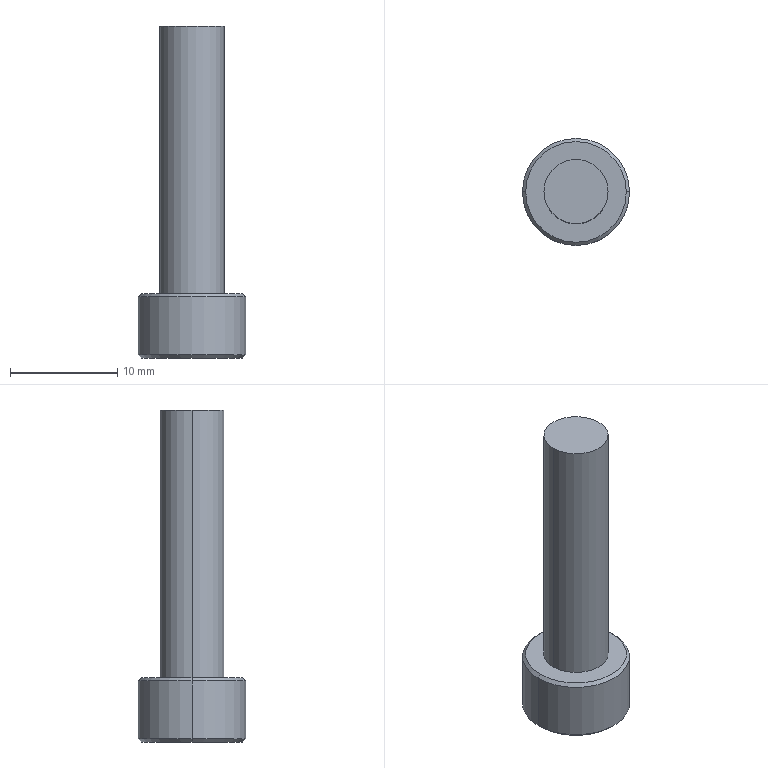Part | SolidWorks | features ICE 2, Chamfer 1, Extrusion 1 | 1 solid | 18 faces | box 10 x 10 x 31 mm | volume 1129 mm3 | plane 10 | cone 4 | cylinder 4 | commonest cylinder face diameters 6 x2 10 x2
STEP:
#1=CARTESIAN_POINT('',(4.7,0.,6.));
#2=VERTEX_POINT('',#1);
#3=CARTESIAN_POINT('',(-4.7,0.,6.));
#4=VERTEX_POINT('',#3);
#5=CARTESIAN_POINT('',(0.,0.,6.));
#6=DIRECTION('',(0.,0.,1.));
#7=DIRECTION('',(1.,0.,0.));
#8=AXIS2_PLACEMENT_3D('',#5,#6,#7);
#9=CIRCLE('',#8,4.7);
#10=EDGE_CURVE('',#2,#4,#9,.T.);
#11=ORIENTED_EDGE('',*,*,#10,.F.);
#12=CARTESIAN_POINT('',(5.,0.,5.7));
#13=VERTEX_POINT('',#12);
#14=CARTESIAN_POINT('',(4.7,0.,6.));
#15=DIRECTION('',(0.7071,0.,-0.7071));
#16=VECTOR('',#15,1000.);
#17=LINE('',#14,#16);
#18=EDGE_CURVE('',#2,#13,#17,.T.);
#19=ORIENTED_EDGE('',*,*,#18,.T.);
#20=CARTESIAN_POINT('',(-5.,0.,5.7));
#21=VERTEX_POINT('',#20);
#22=CARTESIAN_POINT('',(0.,0.,5.7));
#23=DIRECTION('',(0.,0.,-1.));
#24=DIRECTION('',(1.,0.,0.));
#25=AXIS2_PLACEMENT_3D('',#22,#23,#24);
#26=CIRCLE('',#25,5.);
#27=EDGE_CURVE('',#21,#13,#26,.T.);
#28=ORIENTED_EDGE('',*,*,#27,.F.);
#29=CARTESIAN_POINT('',(-4.7,0.,6.));
#30=DIRECTION('',(-0.7071,0.,-0.7071));
#31=VECTOR('',#30,1000.);
#32=LINE('',#29,#31);
#33=EDGE_CURVE('',#4,#21,#32,.T.);
#34=ORIENTED_EDGE('',*,*,#33,.F.);
#35=EDGE_LOOP('',(#11,#19,#28,#34));
#36=FACE_OUTER_BOUND('',#35,.T.);
#37=CARTESIAN_POINT('',(0.,0.,6.));
#38=DIRECTION('',(0.,0.,-1.));
#39=DIRECTION('',(-1.,0.,0.));
#40=AXIS2_PLACEMENT_3D('',#37,#38,#39);
#41=CONICAL_SURFACE('',#40,4.7,0.7854);
#42=ADVANCED_FACE('',(#36),#41,.T.);
#43=CARTESIAN_POINT('',(-4.7,0.,0.));
#44=VERTEX_POINT('',#43);
#45=CARTESIAN_POINT('',(4.7,0.,0.));
#46=VERTEX_POINT('',#45);
#47=CARTESIAN_POINT('',(0.,0.,0.));
#48=DIRECTION('',(0.,0.,-1.));
#49=DIRECTION('',(1.,0.,0.));
#50=AXIS2_PLACEMENT_3D('',#47,#48,#49);
#51=CIRCLE('',#50,4.7);
#52=EDGE_CURVE('',#44,#46,#51,.T.);
#53=ORIENTED_EDGE('',*,*,#52,.F.);
#54=CARTESIAN_POINT('',(-5.,0.,0.3));
#55=VERTEX_POINT('',#54);
#56=CARTESIAN_POINT('',(-5.,0.,0.3));
#57=DIRECTION('',(-0.7071,0.,0.7071));
#58=VECTOR('',#57,1000.);
#59=LINE('',#56,#58);
#60=EDGE_CURVE('',#44,#55,#59,.T.);
#61=ORIENTED_EDGE('',*,*,#60,.T.);
#62=CARTESIAN_POINT('',(5.,0.,0.3));
#63=VERTEX_POINT('',#62);
#64=CARTESIAN_POINT('',(0.,0.,0.3));
#65=DIRECTION('',(0.,0.,1.));
#66=DIRECTION('',(1.,0.,0.));
#67=AXIS2_PLACEMENT_3D('',#64,#65,#66);
#68=CIRCLE('',#67,5.);
#69=EDGE_CURVE('',#63,#55,#68,.T.);
#70=ORIENTED_EDGE('',*,*,#69,.F.);
#71=CARTESIAN_POINT('',(5.,0.,0.3));
#72=DIRECTION('',(0.7071,0.,0.7071));
#73=VECTOR('',#72,1000.);
#74=LINE('',#71,#73);
#75=EDGE_CURVE('',#46,#63,#74,.T.);
#76=ORIENTED_EDGE('',*,*,#75,.F.);
#77=EDGE_LOOP('',(#53,#61,#70,#76));
#78=FACE_OUTER_BOUND('',#77,.T.);
#79=CARTESIAN_POINT('',(0.,0.,0.3));
#80=DIRECTION('',(0.,0.,1.));
#81=DIRECTION('',(1.,0.,0.));
#82=AXIS2_PLACEMENT_3D('',#79,#80,#81);
#83=CONICAL_SURFACE('',#82,5.,0.7854);
#84=ADVANCED_FACE('',(#78),#83,.T.);
#85=CARTESIAN_POINT('',(3.,0.,31.));
#86=VERTEX_POINT('',#85);
#87=CARTESIAN_POINT('',(-3.,0.,31.));
#88=VERTEX_POINT('',#87);
#89=CARTESIAN_POINT('',(0.,0.,31.));
#90=DIRECTION('',(0.,0.,1.));
#91=DIRECTION('',(1.,0.,0.));
#92=AXIS2_PLACEMENT_3D('',#89,#90,#91);
#93=CIRCLE('',#92,3.);
#94=EDGE_CURVE('',#86,#88,#93,.T.);
#95=ORIENTED_EDGE('',*,*,#94,.F.);
#96=CARTESIAN_POINT('',(3.,0.,6.));
#97=VERTEX_POINT('',#96);
#98=CARTESIAN_POINT('',(3.,0.,31.));
#99=DIRECTION('',(0.,0.,-1.));
#100=VECTOR('',#99,1000.);
#101=LINE('',#98,#100);
#102=EDGE_CURVE('',#86,#97,#101,.T.);
#103=ORIENTED_EDGE('',*,*,#102,.T.);
#104=CARTESIAN_POINT('',(-3.,0.,6.));
#105=VERTEX_POINT('',#104);
#106=CARTESIAN_POINT('',(0.,0.,6.));
#107=DIRECTION('',(0.,0.,1.));
#108=DIRECTION('',(1.,0.,0.));
#109=AXIS2_PLACEMENT_3D('',#106,#107,#108);
#110=CIRCLE('',#109,3.);
#111=EDGE_CURVE('',#97,#105,#110,.T.);
#112=ORIENTED_EDGE('',*,*,#111,.T.);
#113=CARTESIAN_POINT('',(-3.,0.,31.));
#114=DIRECTION('',(0.,0.,-1.));
#115=VECTOR('',#114,1000.);
#116=LINE('',#113,#115);
#117=EDGE_CURVE('',#88,#105,#116,.T.);
#118=ORIENTED_EDGE('',*,*,#117,.F.);
#119=EDGE_LOOP('',(#95,#103,#112,#118));
#120=FACE_OUTER_BOUND('',#119,.T.);
#121=CARTESIAN_POINT('',(0.,0.,31.));
#122=DIRECTION('',(0.,0.,-1.));
#123=DIRECTION('',(-1.,0.,0.));
#124=AXIS2_PLACEMENT_3D('',#121,#122,#123);
#125=CYLINDRICAL_SURFACE('',#124,3.);
#126=ADVANCED_FACE('',(#120),#125,.T.);
#127=ORIENTED_EDGE('',*,*,#27,.T.);
#128=CARTESIAN_POINT('',(5.,0.,6.));
#129=DIRECTION('',(0.,0.,-1.));
#130=VECTOR('',#129,1000.);
#131=LINE('',#128,#130);
#132=EDGE_CURVE('',#13,#63,#131,.T.);
#133=ORIENTED_EDGE('',*,*,#132,.T.);
#134=ORIENTED_EDGE('',*,*,#69,.T.);
#135=CARTESIAN_POINT('',(-5.,0.,6.));
#136=DIRECTION('',(0.,0.,-1.));
#137=VECTOR('',#136,1000.);
#138=LINE('',#135,#137);
#139=EDGE_CURVE('',#21,#55,#138,.T.);
#140=ORIENTED_EDGE('',*,*,#139,.F.);
#141=EDGE_LOOP('',(#127,#133,#134,#140));
#142=FACE_OUTER_BOUND('',#141,.T.);
#143=CARTESIAN_POINT('',(0.,0.,6.));
#144=DIRECTION('',(0.,0.,-1.));
#145=DIRECTION('',(-1.,0.,0.));
#146=AXIS2_PLACEMENT_3D('',#143,#144,#145);
#147=CYLINDRICAL_SURFACE('',#146,5.);
#148=ADVANCED_FACE('',(#142),#147,.T.);
#149=ORIENTED_EDGE('',*,*,#132,.F.);
#150=CARTESIAN_POINT('',(0.,0.,5.7));
#151=DIRECTION('',(0.,0.,-1.));
#152=DIRECTION('',(1.,0.,0.));
#153=AXIS2_PLACEMENT_3D('',#150,#151,#152);
#154=CIRCLE('',#153,5.);
#155=EDGE_CURVE('',#13,#21,#154,.T.);
#156=ORIENTED_EDGE('',*,*,#155,.T.);
#157=ORIENTED_EDGE('',*,*,#139,.T.);
#158=CARTESIAN_POINT('',(0.,0.,0.3));
#159=DIRECTION('',(0.,0.,1.));
#160=DIRECTION('',(1.,0.,0.));
#161=AXIS2_PLACEMENT_3D('',#158,#159,#160);
#162=CIRCLE('',#161,5.);
#163=EDGE_CURVE('',#55,#63,#162,.T.);
#164=ORIENTED_EDGE('',*,*,#163,.T.);
#165=EDGE_LOOP('',(#149,#156,#157,#164));
#166=FACE_OUTER_BOUND('',#165,.T.);
#167=CARTESIAN_POINT('',(0.,0.,6.));
#168=DIRECTION('',(0.,0.,-1.));
#169=DIRECTION('',(-1.,0.,0.));
#170=AXIS2_PLACEMENT_3D('',#167,#168,#169);
#171=CYLINDRICAL_SURFACE('',#170,5.);
#172=ADVANCED_FACE('',(#166),#171,.T.);
#173=CARTESIAN_POINT('',(0.,0.,6.));
#174=DIRECTION('',(0.,0.,1.));
#175=DIRECTION('',(1.,0.,0.));
#176=AXIS2_PLACEMENT_3D('',#173,#174,#175);
#177=CIRCLE('',#176,4.7);
#178=EDGE_CURVE('',#4,#2,#177,.T.);
#179=ORIENTED_EDGE('',*,*,#178,.T.);
#180=ORIENTED_EDGE('',*,*,#10,.T.);
#181=EDGE_LOOP('',(#179,#180));
#182=FACE_OUTER_BOUND('',#181,.T.);
#183=CARTESIAN_POINT('',(0.,0.,6.));
#184=DIRECTION('',(0.,0.,1.));
#185=DIRECTION('',(1.,0.,0.));
#186=AXIS2_PLACEMENT_3D('',#183,#184,#185);
#187=CIRCLE('',#186,3.);
#188=EDGE_CURVE('',#105,#97,#187,.T.);
#189=ORIENTED_EDGE('',*,*,#188,.F.);
#190=ORIENTED_EDGE('',*,*,#111,.F.);
#191=EDGE_LOOP('',(#189,#190));
#192=FACE_BOUND('',#191,.T.);
#193=CARTESIAN_POINT('',(0.,0.,6.));
#194=DIRECTION('',(0.,0.,1.));
#195=DIRECTION('',(1.,0.,0.));
#196=AXIS2_PLACEMENT_3D('',#193,#194,#195);
#197=PLANE('',#196);
#198=ADVANCED_FACE('',(#182,#192),#197,.T.);
#199=CARTESIAN_POINT('',(0.,2.429,0.));
#200=VERTEX_POINT('',#199);
#201=CARTESIAN_POINT('',(2.104,1.215,0.));
#202=VERTEX_POINT('',#201);
#203=CARTESIAN_POINT('',(0.,2.429,0.));
#204=DIRECTION('',(0.866,-0.5,0.));
#205=VECTOR('',#204,1000.);
#206=LINE('',#203,#205);
#207=EDGE_CURVE('',#200,#202,#206,.T.);
#208=ORIENTED_EDGE('',*,*,#207,.F.);
#209=CARTESIAN_POINT('',(-2.104,1.215,0.));
#210=VERTEX_POINT('',#209);
#211=CARTESIAN_POINT('',(-2.104,1.215,0.));
#212=DIRECTION('',(0.866,0.5,0.));
#213=VECTOR('',#212,1000.);
#214=LINE('',#211,#213);
#215=EDGE_CURVE('',#210,#200,#214,.T.);
#216=ORIENTED_EDGE('',*,*,#215,.F.);
#217=CARTESIAN_POINT('',(-2.104,-1.215,0.));
#218=VERTEX_POINT('',#217);
#219=CARTESIAN_POINT('',(-2.104,-1.215,0.));
#220=DIRECTION('',(0.,1.,0.));
#221=VECTOR('',#220,1000.);
#222=LINE('',#219,#221);
#223=EDGE_CURVE('',#218,#210,#222,.T.);
#224=ORIENTED_EDGE('',*,*,#223,.F.);
#225=CARTESIAN_POINT('',(0.,-2.429,0.));
#226=VERTEX_POINT('',#225);
#227=CARTESIAN_POINT('',(0.,-2.429,0.));
#228=DIRECTION('',(-0.866,0.5,0.));
#229=VECTOR('',#228,1000.);
#230=LINE('',#227,#229);
#231=EDGE_CURVE('',#226,#218,#230,.T.);
#232=ORIENTED_EDGE('',*,*,#231,.F.);
#233=CARTESIAN_POINT('',(2.104,-1.215,0.));
#234=VERTEX_POINT('',#233);
#235=CARTESIAN_POINT('',(2.104,-1.215,0.));
#236=DIRECTION('',(-0.866,-0.5,0.));
#237=VECTOR('',#236,1000.);
#238=LINE('',#235,#237);
#239=EDGE_CURVE('',#234,#226,#238,.T.);
#240=ORIENTED_EDGE('',*,*,#239,.F.);
#241=CARTESIAN_POINT('',(2.104,1.215,0.));
#242=DIRECTION('',(0.,-1.,0.));
#243=VECTOR('',#242,1000.);
#244=LINE('',#241,#243);
#245=EDGE_CURVE('',#202,#234,#244,.T.);
#246=ORIENTED_EDGE('',*,*,#245,.F.);
#247=EDGE_LOOP('',(#208,#216,#224,#232,#240,#246));
#248=FACE_BOUND('',#247,.T.);
#249=CARTESIAN_POINT('',(0.,0.,0.));
#250=DIRECTION('',(0.,0.,-1.));
#251=DIRECTION('',(1.,0.,0.));
#252=AXIS2_PLACEMENT_3D('',#249,#250,#251);
#253=CIRCLE('',#252,4.7);
#254=EDGE_CURVE('',#46,#44,#253,.T.);
#255=ORIENTED_EDGE('',*,*,#254,.T.);
#256=ORIENTED_EDGE('',*,*,#52,.T.);
#257=EDGE_LOOP('',(#255,#256));
#258=FACE_OUTER_BOUND('',#257,.T.);
#259=CARTESIAN_POINT('',(0.,0.,0.));
#260=DIRECTION('',(0.,0.,1.));
#261=DIRECTION('',(1.,0.,0.));
#262=AXIS2_PLACEMENT_3D('',#259,#260,#261);
#263=PLANE('',#262);
#264=ADVANCED_FACE('',(#248,#258),#263,.F.);
#265=ORIENTED_EDGE('',*,*,#102,.F.);
#266=CARTESIAN_POINT('',(0.,0.,31.));
#267=DIRECTION('',(0.,0.,1.));
#268=DIRECTION('',(1.,0.,0.));
#269=AXIS2_PLACEMENT_3D('',#266,#267,#268);
#270=CIRCLE('',#269,3.);
#271=EDGE_CURVE('',#88,#86,#270,.T.);
#272=ORIENTED_EDGE('',*,*,#271,.F.);
#273=ORIENTED_EDGE('',*,*,#117,.T.);
#274=ORIENTED_EDGE('',*,*,#188,.T.);
#275=EDGE_LOOP('',(#265,#272,#273,#274));
#276=FACE_OUTER_BOUND('',#275,.T.);
#277=CARTESIAN_POINT('',(0.,0.,31.));
#278=DIRECTION('',(0.,0.,-1.));
#279=DIRECTION('',(-1.,0.,0.));
#280=AXIS2_PLACEMENT_3D('',#277,#278,#279);
#281=CYLINDRICAL_SURFACE('',#280,3.);
#282=ADVANCED_FACE('',(#276),#281,.T.);
#283=ORIENTED_EDGE('',*,*,#271,.T.);
#284=ORIENTED_EDGE('',*,*,#94,.T.);
#285=EDGE_LOOP('',(#283,#284));
#286=FACE_OUTER_BOUND('',#285,.T.);
#287=CARTESIAN_POINT('',(0.,0.,31.));
#288=DIRECTION('',(0.,0.,1.));
#289=DIRECTION('',(1.,0.,0.));
#290=AXIS2_PLACEMENT_3D('',#287,#288,#289);
#291=PLANE('',#290);
#292=ADVANCED_FACE('',(#286),#291,.T.);
#293=ORIENTED_EDGE('',*,*,#60,.F.);
#294=ORIENTED_EDGE('',*,*,#254,.F.);
#295=ORIENTED_EDGE('',*,*,#75,.T.);
#296=ORIENTED_EDGE('',*,*,#163,.F.);
#297=EDGE_LOOP('',(#293,#294,#295,#296));
#298=FACE_OUTER_BOUND('',#297,.T.);
#299=CARTESIAN_POINT('',(0.,0.,0.3));
#300=DIRECTION('',(0.,0.,1.));
#301=DIRECTION('',(1.,0.,0.));
#302=AXIS2_PLACEMENT_3D('',#299,#300,#301);
#303=CONICAL_SURFACE('',#302,5.,0.7854);
#304=ADVANCED_FACE('',(#298),#303,.T.);
#305=ORIENTED_EDGE('',*,*,#18,.F.);
#306=ORIENTED_EDGE('',*,*,#178,.F.);
#307=ORIENTED_EDGE('',*,*,#33,.T.);
#308=ORIENTED_EDGE('',*,*,#155,.F.);
#309=EDGE_LOOP('',(#305,#306,#307,#308));
#310=FACE_OUTER_BOUND('',#309,.T.);
#311=CARTESIAN_POINT('',(0.,0.,6.));
#312=DIRECTION('',(0.,0.,-1.));
#313=DIRECTION('',(-1.,0.,0.));
#314=AXIS2_PLACEMENT_3D('',#311,#312,#313);
#315=CONICAL_SURFACE('',#314,4.7,0.7854);
#316=ADVANCED_FACE('',(#310),#315,.T.);
#317=ORIENTED_EDGE('',*,*,#215,.T.);
#318=CARTESIAN_POINT('',(0.,2.429,3.));
#319=VERTEX_POINT('',#318);
#320=CARTESIAN_POINT('',(0.,2.429,3.));
#321=DIRECTION('',(0.,0.,-1.));
#322=VECTOR('',#321,1000.);
#323=LINE('',#320,#322);
#324=EDGE_CURVE('',#319,#200,#323,.T.);
#325=ORIENTED_EDGE('',*,*,#324,.F.);
#326=CARTESIAN_POINT('',(-2.104,1.215,3.));
#327=VERTEX_POINT('',#326);
#328=CARTESIAN_POINT('',(-2.104,1.215,3.));
#329=DIRECTION('',(0.866,0.5,0.));
#330=VECTOR('',#329,1000.);
#331=LINE('',#328,#330);
#332=EDGE_CURVE('',#327,#319,#331,.T.);
#333=ORIENTED_EDGE('',*,*,#332,.F.);
#334=CARTESIAN_POINT('',(-2.104,1.215,3.));
#335=DIRECTION('',(0.,0.,-1.));
#336=VECTOR('',#335,1000.);
#337=LINE('',#334,#336);
#338=EDGE_CURVE('',#327,#210,#337,.T.);
#339=ORIENTED_EDGE('',*,*,#338,.T.);
#340=EDGE_LOOP('',(#317,#325,#333,#339));
#341=FACE_OUTER_BOUND('',#340,.T.);
#342=CARTESIAN_POINT('',(-2.104,1.215,3.));
#343=DIRECTION('',(-0.5,0.866,0.));
#344=DIRECTION('',(-0.866,-0.5,0.));
#345=AXIS2_PLACEMENT_3D('',#342,#343,#344);
#346=PLANE('',#345);
#347=ADVANCED_FACE('',(#341),#346,.F.);
#348=ORIENTED_EDGE('',*,*,#223,.T.);
#349=ORIENTED_EDGE('',*,*,#338,.F.);
#350=CARTESIAN_POINT('',(-2.104,-1.215,3.));
#351=VERTEX_POINT('',#350);
#352=CARTESIAN_POINT('',(-2.104,-1.215,3.));
#353=DIRECTION('',(0.,1.,0.));
#354=VECTOR('',#353,1000.);
#355=LINE('',#352,#354);
#356=EDGE_CURVE('',#351,#327,#355,.T.);
#357=ORIENTED_EDGE('',*,*,#356,.F.);
#358=CARTESIAN_POINT('',(-2.104,-1.215,3.));
#359=DIRECTION('',(0.,0.,-1.));
#360=VECTOR('',#359,1000.);
#361=LINE('',#358,#360);
#362=EDGE_CURVE('',#351,#218,#361,.T.);
#363=ORIENTED_EDGE('',*,*,#362,.T.);
#364=EDGE_LOOP('',(#348,#349,#357,#363));
#365=FACE_OUTER_BOUND('',#364,.T.);
#366=CARTESIAN_POINT('',(-2.104,-1.215,3.));
#367=DIRECTION('',(-1.,0.,0.));
#368=DIRECTION('',(0.,-1.,0.));
#369=AXIS2_PLACEMENT_3D('',#366,#367,#368);
#370=PLANE('',#369);
#371=ADVANCED_FACE('',(#365),#370,.F.);
#372=ORIENTED_EDGE('',*,*,#231,.T.);
#373=ORIENTED_EDGE('',*,*,#362,.F.);
#374=CARTESIAN_POINT('',(0.,-2.429,3.));
#375=VERTEX_POINT('',#374);
#376=CARTESIAN_POINT('',(0.,-2.429,3.));
#377=DIRECTION('',(-0.866,0.5,0.));
#378=VECTOR('',#377,1000.);
#379=LINE('',#376,#378);
#380=EDGE_CURVE('',#375,#351,#379,.T.);
#381=ORIENTED_EDGE('',*,*,#380,.F.);
#382=CARTESIAN_POINT('',(0.,-2.429,3.));
#383=DIRECTION('',(0.,0.,-1.));
#384=VECTOR('',#383,1000.);
#385=LINE('',#382,#384);
#386=EDGE_CURVE('',#375,#226,#385,.T.);
#387=ORIENTED_EDGE('',*,*,#386,.T.);
#388=EDGE_LOOP('',(#372,#373,#381,#387));
#389=FACE_OUTER_BOUND('',#388,.T.);
#390=CARTESIAN_POINT('',(0.,-2.429,3.));
#391=DIRECTION('',(-0.5,-0.866,0.));
#392=DIRECTION('',(0.866,-0.5,0.));
#393=AXIS2_PLACEMENT_3D('',#390,#391,#392);
#394=PLANE('',#393);
#395=ADVANCED_FACE('',(#389),#394,.F.);
#396=ORIENTED_EDGE('',*,*,#239,.T.);
#397=ORIENTED_EDGE('',*,*,#386,.F.);
#398=CARTESIAN_POINT('',(2.104,-1.215,3.));
#399=VERTEX_POINT('',#398);
#400=CARTESIAN_POINT('',(2.104,-1.215,3.));
#401=DIRECTION('',(-0.866,-0.5,0.));
#402=VECTOR('',#401,1000.);
#403=LINE('',#400,#402);
#404=EDGE_CURVE('',#399,#375,#403,.T.);
#405=ORIENTED_EDGE('',*,*,#404,.F.);
#406=CARTESIAN_POINT('',(2.104,-1.215,3.));
#407=DIRECTION('',(0.,0.,-1.));
#408=VECTOR('',#407,1000.);
#409=LINE('',#406,#408);
#410=EDGE_CURVE('',#399,#234,#409,.T.);
#411=ORIENTED_EDGE('',*,*,#410,.T.);
#412=EDGE_LOOP('',(#396,#397,#405,#411));
#413=FACE_OUTER_BOUND('',#412,.T.);
#414=CARTESIAN_POINT('',(2.104,-1.215,3.));
#415=DIRECTION('',(0.5,-0.866,0.));
#416=DIRECTION('',(0.866,0.5,0.));
#417=AXIS2_PLACEMENT_3D('',#414,#415,#416);
#418=PLANE('',#417);
#419=ADVANCED_FACE('',(#413),#418,.F.);
#420=ORIENTED_EDGE('',*,*,#245,.T.);
#421=ORIENTED_EDGE('',*,*,#410,.F.);
#422=CARTESIAN_POINT('',(2.104,1.215,3.));
#423=VERTEX_POINT('',#422);
#424=CARTESIAN_POINT('',(2.104,1.215,3.));
#425=DIRECTION('',(0.,-1.,0.));
#426=VECTOR('',#425,1000.);
#427=LINE('',#424,#426);
#428=EDGE_CURVE('',#423,#399,#427,.T.);
#429=ORIENTED_EDGE('',*,*,#428,.F.);
#430=CARTESIAN_POINT('',(2.104,1.215,3.));
#431=DIRECTION('',(0.,0.,-1.));
#432=VECTOR('',#431,1000.);
#433=LINE('',#430,#432);
#434=EDGE_CURVE('',#423,#202,#433,.T.);
#435=ORIENTED_EDGE('',*,*,#434,.T.);
#436=EDGE_LOOP('',(#420,#421,#429,#435));
#437=FACE_OUTER_BOUND('',#436,.T.);
#438=CARTESIAN_POINT('',(2.104,1.215,3.));
#439=DIRECTION('',(1.,0.,0.));
#440=DIRECTION('',(0.,1.,0.));
#441=AXIS2_PLACEMENT_3D('',#438,#439,#440);
#442=PLANE('',#441);
#443=ADVANCED_FACE('',(#437),#442,.F.);
#444=ORIENTED_EDGE('',*,*,#207,.T.);
#445=ORIENTED_EDGE('',*,*,#434,.F.);
#446=CARTESIAN_POINT('',(0.,2.429,3.));
#447=DIRECTION('',(0.866,-0.5,0.));
#448=VECTOR('',#447,1000.);
#449=LINE('',#446,#448);
#450=EDGE_CURVE('',#319,#423,#449,.T.);
#451=ORIENTED_EDGE('',*,*,#450,.F.);
#452=ORIENTED_EDGE('',*,*,#324,.T.);
#453=EDGE_LOOP('',(#444,#445,#451,#452));
#454=FACE_OUTER_BOUND('',#453,.T.);
#455=CARTESIAN_POINT('',(0.,2.429,3.));
#456=DIRECTION('',(0.5,0.866,0.));
#457=DIRECTION('',(-0.866,0.5,0.));
#458=AXIS2_PLACEMENT_3D('',#455,#456,#457);
#459=PLANE('',#458);
#460=ADVANCED_FACE('',(#454),#459,.F.);
#461=ORIENTED_EDGE('',*,*,#332,.T.);
#462=ORIENTED_EDGE('',*,*,#450,.T.);
#463=ORIENTED_EDGE('',*,*,#428,.T.);
#464=ORIENTED_EDGE('',*,*,#404,.T.);
#465=ORIENTED_EDGE('',*,*,#380,.T.);
#466=ORIENTED_EDGE('',*,*,#356,.T.);
#467=EDGE_LOOP('',(#461,#462,#463,#464,#465,#466));
#468=FACE_OUTER_BOUND('',#467,.T.);
#469=CARTESIAN_POINT('',(0.,0.,3.));
#470=DIRECTION('',(0.,0.,-1.));
#471=DIRECTION('',(-1.,0.,0.));
#472=AXIS2_PLACEMENT_3D('',#469,#470,#471);
#473=PLANE('',#472);
#474=ADVANCED_FACE('',(#468),#473,.T.);
#475=CLOSED_SHELL('',(#42,#84,#126,#148,#172,#198,#264,#282,#292,#304,#316,#347,#371,#395,#419,#443,#460,#474));
#476=MANIFOLD_SOLID_BREP('',#475);
#477=CARTESIAN_POINT('',(0.,0.,0.));
#478=DIRECTION('',(0.,0.,1.));
#479=DIRECTION('',(1.,0.,0.));
#480=AXIS2_PLACEMENT_3D('',#477,#478,#479);
#481=(LENGTH_UNIT()NAMED_UNIT(*)SI_UNIT(.MILLI.,.METRE.));
#482=UNCERTAINTY_MEASURE_WITH_UNIT(LENGTH_MEASURE(0.00001),#481,'','');
#483=(NAMED_UNIT(*)PLANE_ANGLE_UNIT()SI_UNIT($,.RADIAN.));
#484=(NAMED_UNIT(*)SI_UNIT($,.STERADIAN.)SOLID_ANGLE_UNIT());
#485=(GEOMETRIC_REPRESENTATION_CONTEXT(3)GLOBAL_UNCERTAINTY_ASSIGNED_CONTEXT((#482))GLOBAL_UNIT_ASSIGNED_CONTEXT((#481,#483,#484))REPRESENTATION_CONTEXT('',''));
#486=ADVANCED_BREP_SHAPE_REPRESENTATION('',(#476,#480),#485);